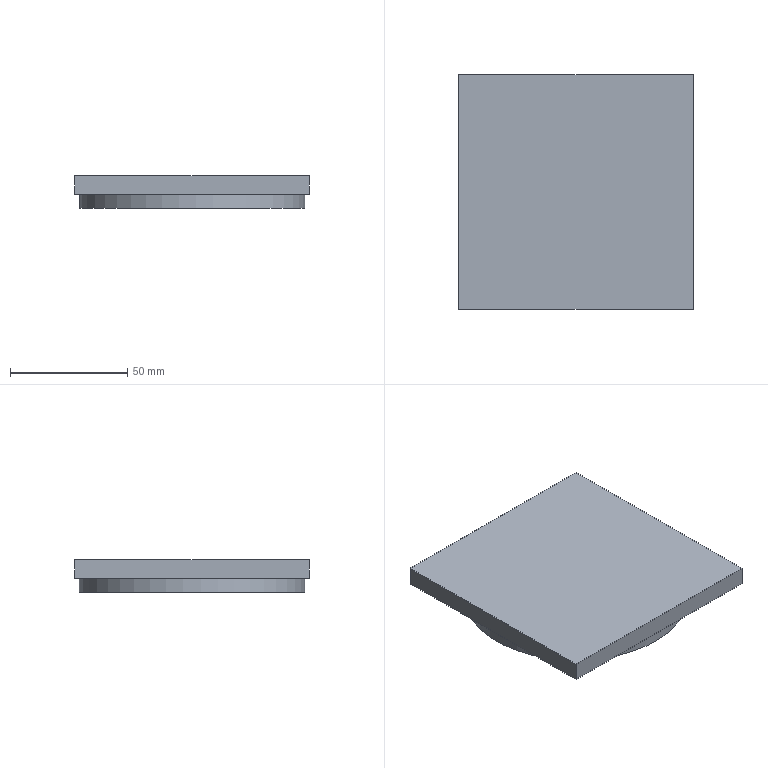NC program | NX | posted with a generic post | part box 100 x 100 x 14 mm
Lines 1666 to 1798 of 1798:
(PLANAR_MILL_2 , TOOL : SPOTDRILL-D8)
N3294 T04 M6
N3296 G53
N3298 G17 G0 G90 X-53.963 Y-2. S3000 M3
N3300 G43 Z50. H4
N3302 Z1.
N3304 G94 G1 Z-2. F1500.
N3306 X-52.
N3308 G3 X-50. Y0. R2.
N3310 G2 X0. Y50. R50.
N3312 X-50. Y0. R-50.
N3314 G3 X-52. Y2. R2.
N3316 G1 X-53.963
N3318 Z1.
N3320 G0 Z50.
(PLANAR_MILL_2_COPY , TOOL : SPOTDRILL-D8)
N3322 X-23.85 Y-35.113
N3324 Z1.5
N3326 G1 Z-1.5 F500.
N3328 G3 X-24.85 Y-36.113 R1.
N3330 X-20.85 Y-40.113 R4.
N3332 X-24.85 Y-36.113 R-4.
N3334 X-23.85 Y-37.113 R1.
N3336 G1 Z1.5
N3338 G0 Z50.
N3340 X-17.85 Y35.113
N3342 Z1.5
N3344 G1 Z-1.5
N3346 G3 X-16.85 Y36.113 R1.
N3348 X-20.85 Y40.113 R4.
N3350 X-16.85 Y36.113 R-4.
N3352 X-17.85 Y37.113 R1.
N3354 G1 Z1.5
N3356 G0 Z50.
N3358 X38.7 Y1.
N3360 Z1.5
N3362 G1 Z-1.5
N3364 G3 X37.7 Y0. R1.
N3366 X41.7 Y-4. R4.
N3368 X37.7 Y0. R-4.
N3370 X38.7 Y-1. R1.
N3372 G1 Z1.5
N3374 G0 Z50.
(PLANAR_MILL_2_COPY_COPY , TOOL : SPOTDRILL-D8)
N3376 X-21.65 Y1.
N3378 Z1.5
N3380 G1 Z-1.5
N3382 G3 X-22.65 Y0. R1.
N3384 X0. Y-22.65 R22.65
N3386 X-22.65 Y0. R-22.65
N3388 X-21.65 Y-1. R1.
N3390 G1 Z1.5
N3392 G0 Z50.
N3394 M5
(PLANAR_MILL_COPY , TOOL : D-6)
N3396 T03 M6
N3398 G53
N3400 G17 G0 G90 X-22.35 Y-35.113 S4500 M3
N3402 G43 Z50. H3
N3404 Z0.
N3406 G94 G1 Z-3. F200.
N3408 G3 X-23.35 Y-36.113 R1.
N3410 X-20.85 Y-38.613 R2.5
N3412 X-23.35 Y-36.113 R-2.5
N3414 X-22.35 Y-37.113 R1.
N3416 G1 Z0.
N3418 G0 Z50.
N3420 X-19.35 Y35.113
N3422 Z0.
N3424 G1 Z-3.
N3426 G3 X-18.35 Y36.113 R1.
N3428 X-20.85 Y38.613 R2.5
N3430 X-18.35 Y36.113 R-2.5
N3432 X-19.35 Y37.113 R1.
N3434 G1 Z0.
N3436 G0 Z50.
N3438 X40.2 Y1.
N3440 Z0.
N3442 G1 Z-3.
N3444 G3 X39.2 Y0. R1.
N3446 X41.7 Y-2.5 R2.5
N3448 X39.2 Y0. R-2.5
N3450 X40.2 Y-1. R1.
N3452 G1 Z0.
N3454 G0 Z50.
N3456 M5
(PLANAR_MILL_1 , TOOL : D10)
N3458 T07 M6
N3460 G53
N3462 G17 G0 G90 X-58.95 Y-1.826 S4500 M3
N3464 G43 Z50. H7
N3466 Z-4.
N3468 G94 G1 Z-7. F1000.
N3470 G41 X-57.966 Y-2. D7
N3472 X-55.
N3474 G3 X-53. Y0. R2.
N3476 G2 X0. Y53. R53.
N3478 X-53. Y0. R-53.
N3480 G3 X-55. Y2. R2.
N3482 G1 X-57.966
N3484 G40
N3486 X-58.95 Y1.826
N3488 Z-4.
N3490 G0 Z50.
(PLANAR_MILL_1_COPY , TOOL : D10)
N3492 X-13.023
N3494 Z-4.
N3496 G1 Z-7.
N3498 G41 X-14.008 Y2.
N3500 X-17.15
N3502 G3 X-19.15 Y0. R2.
N3504 X0. Y-19.15 R19.15
N3506 X-19.15 Y0. R-19.15
N3508 X-17.15 Y-2. R2.
N3510 G1 X-14.008
N3512 G40
N3514 X-13.023 Y-1.826
N3516 Z-4.
N3518 G0 Z50.
N3520 M5
N3522 M2